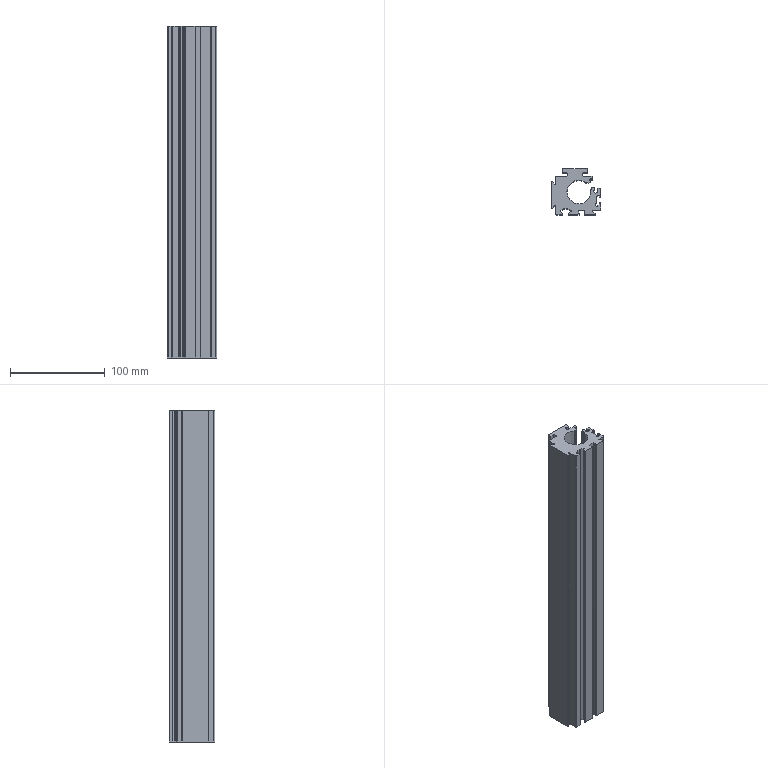Part | STEP file | DGC-25 cylinder body_DGC-25-200-G-PPV-A | 1 solid | 137 faces | box 52.1 x 48.5 x 351 mm | volume 492103 mm3 | cylinder 72 | plane 65 | commonest cylinder face diameters 0.4 x19 1 x11 2 x10 0.6 x6 0.8 x6 1.5 x6